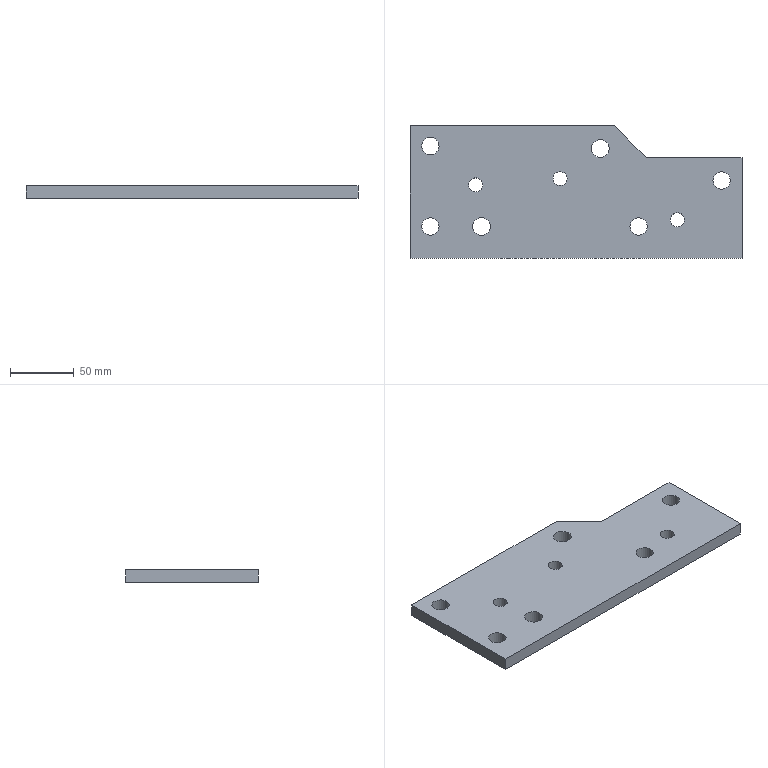Part | STEP file | lll_id114_x_t | 1 solid | 17 faces | box 260 x 104 x 10 mm | volume 236864 mm3 | cylinder 9 | plane 8 | commonest cylinder face diameters 11 x3 13.509 x3 14 x2 13.5 x1
STEP:
#1=CARTESIAN_POINT('',(832.25,-19.75,92.5));
#2=VERTEX_POINT('',#1);
#3=CARTESIAN_POINT('',(825.5,-19.75,92.5));
#4=DIRECTION('',(0.,0.,1.));
#5=DIRECTION('',(1.,0.,0.));
#6=AXIS2_PLACEMENT_3D('',#3,#4,#5);
#7=CIRCLE('',#6,6.75);
#8=EDGE_CURVE('',#2,#2,#7,.T.);
#9=ORIENTED_EDGE('',*,*,#8,.T.);
#10=EDGE_LOOP('',(#9));
#11=FACE_BOUND('',#10,.T.);
#12=CARTESIAN_POINT('',(741.5,23.25,92.5));
#13=VERTEX_POINT('',#12);
#14=CARTESIAN_POINT('',(766.5,-1.75,92.5));
#15=VERTEX_POINT('',#14);
#16=CARTESIAN_POINT('',(734.,30.75,92.5));
#17=DIRECTION('',(0.7071,-0.7071,0.));
#18=VECTOR('',#17,1.);
#19=LINE('',#16,#18);
#20=EDGE_CURVE('',#13,#15,#19,.T.);
#21=ORIENTED_EDGE('',*,*,#20,.T.);
#22=CARTESIAN_POINT('',(841.5,-1.75,92.5));
#23=VERTEX_POINT('',#22);
#24=CARTESIAN_POINT('',(841.5,-1.75,92.5));
#25=DIRECTION('',(-1.,0.,0.));
#26=VECTOR('',#25,1.);
#27=LINE('',#24,#26);
#28=EDGE_CURVE('',#23,#15,#27,.T.);
#29=ORIENTED_EDGE('',*,*,#28,.F.);
#30=CARTESIAN_POINT('',(841.5,-80.75,92.5));
#31=VERTEX_POINT('',#30);
#32=CARTESIAN_POINT('',(841.5,-1.75,92.5));
#33=DIRECTION('',(0.,-1.,0.));
#34=VECTOR('',#33,1.);
#35=LINE('',#32,#34);
#36=EDGE_CURVE('',#23,#31,#35,.T.);
#37=ORIENTED_EDGE('',*,*,#36,.T.);
#38=CARTESIAN_POINT('',(581.5,-80.75,92.5));
#39=VERTEX_POINT('',#38);
#40=CARTESIAN_POINT('',(679.,-80.75,92.5));
#41=DIRECTION('',(1.,0.,0.));
#42=VECTOR('',#41,1.);
#43=LINE('',#40,#42);
#44=EDGE_CURVE('',#39,#31,#43,.T.);
#45=ORIENTED_EDGE('',*,*,#44,.F.);
#46=CARTESIAN_POINT('',(581.5,23.25,92.5));
#47=VERTEX_POINT('',#46);
#48=CARTESIAN_POINT('',(581.5,-24.25,92.5));
#49=DIRECTION('',(0.,-1.,0.));
#50=VECTOR('',#49,1.);
#51=LINE('',#48,#50);
#52=EDGE_CURVE('',#47,#39,#51,.T.);
#53=ORIENTED_EDGE('',*,*,#52,.F.);
#54=CARTESIAN_POINT('',(679.,23.25,92.5));
#55=DIRECTION('',(-1.,0.,0.));
#56=VECTOR('',#55,1.);
#57=LINE('',#54,#56);
#58=EDGE_CURVE('',#13,#47,#57,.T.);
#59=ORIENTED_EDGE('',*,*,#58,.F.);
#60=EDGE_LOOP('',(#21,#29,#37,#45,#53,#59));
#61=FACE_BOUND('',#60,.T.);
#62=CARTESIAN_POINT('',(693.5,-18.25,92.5));
#63=VERTEX_POINT('',#62);
#64=CARTESIAN_POINT('',(699.,-18.25,92.5));
#65=DIRECTION('',(0.,0.,1.));
#66=DIRECTION('',(-1.,0.,0.));
#67=AXIS2_PLACEMENT_3D('',#64,#65,#66);
#68=CIRCLE('',#67,5.5);
#69=EDGE_CURVE('',#63,#63,#68,.T.);
#70=ORIENTED_EDGE('',*,*,#69,.T.);
#71=EDGE_LOOP('',(#70));
#72=FACE_BOUND('',#71,.T.);
#73=CARTESIAN_POINT('',(723.5,5.25,92.5));
#74=VERTEX_POINT('',#73);
#75=CARTESIAN_POINT('',(730.5,5.25,92.5));
#76=DIRECTION('',(0.,0.,1.));
#77=DIRECTION('',(-1.,0.,0.));
#78=AXIS2_PLACEMENT_3D('',#75,#76,#77);
#79=CIRCLE('',#78,7.);
#80=EDGE_CURVE('',#74,#74,#79,.T.);
#81=ORIENTED_EDGE('',*,*,#80,.T.);
#82=EDGE_LOOP('',(#81));
#83=FACE_BOUND('',#82,.T.);
#84=CARTESIAN_POINT('',(590.745,7.25,92.5));
#85=VERTEX_POINT('',#84);
#86=CARTESIAN_POINT('',(597.5,7.25,92.5));
#87=DIRECTION('',(0.,0.,1.));
#88=DIRECTION('',(-1.,0.,0.));
#89=AXIS2_PLACEMENT_3D('',#86,#87,#88);
#90=CIRCLE('',#89,6.755);
#91=EDGE_CURVE('',#85,#85,#90,.T.);
#92=ORIENTED_EDGE('',*,*,#91,.T.);
#93=EDGE_LOOP('',(#92));
#94=FACE_BOUND('',#93,.T.);
#95=CARTESIAN_POINT('',(590.745,-55.75,92.5));
#96=VERTEX_POINT('',#95);
#97=CARTESIAN_POINT('',(597.5,-55.75,92.5));
#98=DIRECTION('',(0.,0.,1.));
#99=DIRECTION('',(-1.,0.,0.));
#100=AXIS2_PLACEMENT_3D('',#97,#98,#99);
#101=CIRCLE('',#100,6.755);
#102=EDGE_CURVE('',#96,#96,#101,.T.);
#103=ORIENTED_EDGE('',*,*,#102,.T.);
#104=EDGE_LOOP('',(#103));
#105=FACE_BOUND('',#104,.T.);
#106=CARTESIAN_POINT('',(753.745,-55.75,92.5));
#107=VERTEX_POINT('',#106);
#108=CARTESIAN_POINT('',(760.5,-55.75,92.5));
#109=DIRECTION('',(0.,0.,1.));
#110=DIRECTION('',(-1.,0.,0.));
#111=AXIS2_PLACEMENT_3D('',#108,#109,#110);
#112=CIRCLE('',#111,6.755);
#113=EDGE_CURVE('',#107,#107,#112,.T.);
#114=ORIENTED_EDGE('',*,*,#113,.T.);
#115=EDGE_LOOP('',(#114));
#116=FACE_BOUND('',#115,.T.);
#117=CARTESIAN_POINT('',(630.5,-55.75,92.5));
#118=VERTEX_POINT('',#117);
#119=CARTESIAN_POINT('',(637.5,-55.75,92.5));
#120=DIRECTION('',(0.,0.,1.));
#121=DIRECTION('',(-1.,0.,0.));
#122=AXIS2_PLACEMENT_3D('',#119,#120,#121);
#123=CIRCLE('',#122,7.);
#124=EDGE_CURVE('',#118,#118,#123,.T.);
#125=ORIENTED_EDGE('',*,*,#124,.T.);
#126=EDGE_LOOP('',(#125));
#127=FACE_BOUND('',#126,.T.);
#128=CARTESIAN_POINT('',(627.5,-23.25,92.5));
#129=VERTEX_POINT('',#128);
#130=CARTESIAN_POINT('',(633.,-23.25,92.5));
#131=DIRECTION('',(0.,0.,1.));
#132=DIRECTION('',(-1.,0.,0.));
#133=AXIS2_PLACEMENT_3D('',#130,#131,#132);
#134=CIRCLE('',#133,5.5);
#135=EDGE_CURVE('',#129,#129,#134,.T.);
#136=ORIENTED_EDGE('',*,*,#135,.T.);
#137=EDGE_LOOP('',(#136));
#138=FACE_BOUND('',#137,.T.);
#139=CARTESIAN_POINT('',(796.273,-50.5,92.5));
#140=VERTEX_POINT('',#139);
#141=CARTESIAN_POINT('',(790.773,-50.5,92.5));
#142=DIRECTION('',(0.,0.,1.));
#143=DIRECTION('',(1.,0.,0.));
#144=AXIS2_PLACEMENT_3D('',#141,#142,#143);
#145=CIRCLE('',#144,5.5);
#146=EDGE_CURVE('',#140,#140,#145,.T.);
#147=ORIENTED_EDGE('',*,*,#146,.T.);
#148=EDGE_LOOP('',(#147));
#149=FACE_BOUND('',#148,.T.);
#150=CARTESIAN_POINT('',(679.,-24.25,92.5));
#151=DIRECTION('',(0.,0.,-1.));
#152=DIRECTION('',(1.,0.,0.));
#153=AXIS2_PLACEMENT_3D('',#150,#151,#152);
#154=PLANE('',#153);
#155=ADVANCED_FACE('',(#11,#61,#72,#83,#94,#105,#116,#127,#138,#149),#154,.T.);
#156=CARTESIAN_POINT('',(581.5,23.25,102.5));
#157=VERTEX_POINT('',#156);
#158=CARTESIAN_POINT('',(741.5,23.25,102.5));
#159=VERTEX_POINT('',#158);
#160=CARTESIAN_POINT('',(679.,23.25,102.5));
#161=DIRECTION('',(1.,0.,0.));
#162=VECTOR('',#161,1.);
#163=LINE('',#160,#162);
#164=EDGE_CURVE('',#157,#159,#163,.T.);
#165=ORIENTED_EDGE('',*,*,#164,.T.);
#166=CARTESIAN_POINT('',(741.5,23.25,92.5));
#167=DIRECTION('',(0.,0.,-1.));
#168=VECTOR('',#167,1.);
#169=LINE('',#166,#168);
#170=EDGE_CURVE('',#159,#13,#169,.T.);
#171=ORIENTED_EDGE('',*,*,#170,.T.);
#172=ORIENTED_EDGE('',*,*,#58,.T.);
#173=CARTESIAN_POINT('',(581.5,23.25,92.5));
#174=DIRECTION('',(0.,0.,1.));
#175=VECTOR('',#174,1.);
#176=LINE('',#173,#175);
#177=EDGE_CURVE('',#47,#157,#176,.T.);
#178=ORIENTED_EDGE('',*,*,#177,.T.);
#179=EDGE_LOOP('',(#165,#171,#172,#178));
#180=FACE_OUTER_BOUND('',#179,.T.);
#181=CARTESIAN_POINT('',(679.,23.25,92.5));
#182=DIRECTION('',(0.,1.,0.));
#183=DIRECTION('',(0.,0.,-1.));
#184=AXIS2_PLACEMENT_3D('',#181,#182,#183);
#185=PLANE('',#184);
#186=ADVANCED_FACE('',(#180),#185,.T.);
#187=CARTESIAN_POINT('',(841.5,-80.75,102.5));
#188=VERTEX_POINT('',#187);
#189=CARTESIAN_POINT('',(581.5,-80.75,102.5));
#190=VERTEX_POINT('',#189);
#191=CARTESIAN_POINT('',(741.5,-80.75,102.5));
#192=DIRECTION('',(-1.,0.,0.));
#193=VECTOR('',#192,1.);
#194=LINE('',#191,#193);
#195=EDGE_CURVE('',#188,#190,#194,.T.);
#196=ORIENTED_EDGE('',*,*,#195,.T.);
#197=CARTESIAN_POINT('',(581.5,-80.75,92.5));
#198=DIRECTION('',(0.,0.,1.));
#199=VECTOR('',#198,1.);
#200=LINE('',#197,#199);
#201=EDGE_CURVE('',#39,#190,#200,.T.);
#202=ORIENTED_EDGE('',*,*,#201,.F.);
#203=ORIENTED_EDGE('',*,*,#44,.T.);
#204=CARTESIAN_POINT('',(841.5,-80.75,102.5));
#205=DIRECTION('',(0.,0.,-1.));
#206=VECTOR('',#205,1.);
#207=LINE('',#204,#206);
#208=EDGE_CURVE('',#188,#31,#207,.T.);
#209=ORIENTED_EDGE('',*,*,#208,.F.);
#210=EDGE_LOOP('',(#196,#202,#203,#209));
#211=FACE_OUTER_BOUND('',#210,.T.);
#212=CARTESIAN_POINT('',(679.,-80.75,92.5));
#213=DIRECTION('',(0.,-1.,0.));
#214=DIRECTION('',(0.,0.,1.));
#215=AXIS2_PLACEMENT_3D('',#212,#213,#214);
#216=PLANE('',#215);
#217=ADVANCED_FACE('',(#211),#216,.T.);
#218=CARTESIAN_POINT('',(581.5,-24.25,102.5));
#219=DIRECTION('',(0.,-1.,0.));
#220=VECTOR('',#219,1.);
#221=LINE('',#218,#220);
#222=EDGE_CURVE('',#157,#190,#221,.T.);
#223=ORIENTED_EDGE('',*,*,#222,.F.);
#224=ORIENTED_EDGE('',*,*,#177,.F.);
#225=ORIENTED_EDGE('',*,*,#52,.T.);
#226=ORIENTED_EDGE('',*,*,#201,.T.);
#227=EDGE_LOOP('',(#223,#224,#225,#226));
#228=FACE_OUTER_BOUND('',#227,.T.);
#229=CARTESIAN_POINT('',(581.5,-24.25,92.5));
#230=DIRECTION('',(-1.,0.,0.));
#231=DIRECTION('',(0.,0.,-1.));
#232=AXIS2_PLACEMENT_3D('',#229,#230,#231);
#233=PLANE('',#232);
#234=ADVANCED_FACE('',(#228),#233,.T.);
#235=CARTESIAN_POINT('',(590.745,-55.75,102.5));
#236=VERTEX_POINT('',#235);
#237=CARTESIAN_POINT('',(597.5,-55.75,102.5));
#238=DIRECTION('',(0.,0.,1.));
#239=DIRECTION('',(-1.,0.,0.));
#240=AXIS2_PLACEMENT_3D('',#237,#238,#239);
#241=CIRCLE('',#240,6.755);
#242=EDGE_CURVE('',#236,#236,#241,.T.);
#243=ORIENTED_EDGE('',*,*,#242,.T.);
#244=EDGE_LOOP('',(#243));
#245=FACE_BOUND('',#244,.T.);
#246=ORIENTED_EDGE('',*,*,#102,.F.);
#247=EDGE_LOOP('',(#246));
#248=FACE_BOUND('',#247,.T.);
#249=CARTESIAN_POINT('',(597.5,-55.75,92.5));
#250=DIRECTION('',(0.,0.,1.));
#251=DIRECTION('',(-1.,0.,0.));
#252=AXIS2_PLACEMENT_3D('',#249,#250,#251);
#253=CYLINDRICAL_SURFACE('',#252,6.755);
#254=ADVANCED_FACE('',(#245,#248),#253,.F.);
#255=CARTESIAN_POINT('',(590.745,7.25,102.5));
#256=VERTEX_POINT('',#255);
#257=CARTESIAN_POINT('',(597.5,7.25,102.5));
#258=DIRECTION('',(0.,0.,1.));
#259=DIRECTION('',(-1.,0.,0.));
#260=AXIS2_PLACEMENT_3D('',#257,#258,#259);
#261=CIRCLE('',#260,6.755);
#262=EDGE_CURVE('',#256,#256,#261,.T.);
#263=ORIENTED_EDGE('',*,*,#262,.T.);
#264=EDGE_LOOP('',(#263));
#265=FACE_BOUND('',#264,.T.);
#266=ORIENTED_EDGE('',*,*,#91,.F.);
#267=EDGE_LOOP('',(#266));
#268=FACE_BOUND('',#267,.T.);
#269=CARTESIAN_POINT('',(597.5,7.25,92.5));
#270=DIRECTION('',(0.,0.,1.));
#271=DIRECTION('',(-1.,0.,0.));
#272=AXIS2_PLACEMENT_3D('',#269,#270,#271);
#273=CYLINDRICAL_SURFACE('',#272,6.755);
#274=ADVANCED_FACE('',(#265,#268),#273,.F.);
#275=CARTESIAN_POINT('',(753.745,-55.75,102.5));
#276=VERTEX_POINT('',#275);
#277=CARTESIAN_POINT('',(760.5,-55.75,102.5));
#278=DIRECTION('',(0.,0.,1.));
#279=DIRECTION('',(-1.,0.,0.));
#280=AXIS2_PLACEMENT_3D('',#277,#278,#279);
#281=CIRCLE('',#280,6.755);
#282=EDGE_CURVE('',#276,#276,#281,.T.);
#283=ORIENTED_EDGE('',*,*,#282,.T.);
#284=EDGE_LOOP('',(#283));
#285=FACE_BOUND('',#284,.T.);
#286=ORIENTED_EDGE('',*,*,#113,.F.);
#287=EDGE_LOOP('',(#286));
#288=FACE_BOUND('',#287,.T.);
#289=CARTESIAN_POINT('',(760.5,-55.75,92.5));
#290=DIRECTION('',(0.,0.,1.));
#291=DIRECTION('',(-1.,0.,0.));
#292=AXIS2_PLACEMENT_3D('',#289,#290,#291);
#293=CYLINDRICAL_SURFACE('',#292,6.755);
#294=ADVANCED_FACE('',(#285,#288),#293,.F.);
#295=CARTESIAN_POINT('',(723.5,5.25,102.5));
#296=VERTEX_POINT('',#295);
#297=CARTESIAN_POINT('',(730.5,5.25,102.5));
#298=DIRECTION('',(0.,0.,-1.));
#299=DIRECTION('',(-1.,0.,0.));
#300=AXIS2_PLACEMENT_3D('',#297,#298,#299);
#301=CIRCLE('',#300,7.);
#302=EDGE_CURVE('',#296,#296,#301,.T.);
#303=ORIENTED_EDGE('',*,*,#302,.F.);
#304=EDGE_LOOP('',(#303));
#305=FACE_BOUND('',#304,.T.);
#306=ORIENTED_EDGE('',*,*,#80,.F.);
#307=EDGE_LOOP('',(#306));
#308=FACE_BOUND('',#307,.T.);
#309=CARTESIAN_POINT('',(730.5,5.25,92.5));
#310=DIRECTION('',(0.,0.,1.));
#311=DIRECTION('',(-1.,0.,0.));
#312=AXIS2_PLACEMENT_3D('',#309,#310,#311);
#313=CYLINDRICAL_SURFACE('',#312,7.);
#314=ADVANCED_FACE('',(#305,#308),#313,.F.);
#315=CARTESIAN_POINT('',(630.5,-55.75,102.5));
#316=VERTEX_POINT('',#315);
#317=CARTESIAN_POINT('',(637.5,-55.75,102.5));
#318=DIRECTION('',(0.,0.,1.));
#319=DIRECTION('',(-1.,0.,0.));
#320=AXIS2_PLACEMENT_3D('',#317,#318,#319);
#321=CIRCLE('',#320,7.);
#322=EDGE_CURVE('',#316,#316,#321,.T.);
#323=ORIENTED_EDGE('',*,*,#322,.T.);
#324=EDGE_LOOP('',(#323));
#325=FACE_BOUND('',#324,.T.);
#326=ORIENTED_EDGE('',*,*,#124,.F.);
#327=EDGE_LOOP('',(#326));
#328=FACE_BOUND('',#327,.T.);
#329=CARTESIAN_POINT('',(637.5,-55.75,92.5));
#330=DIRECTION('',(0.,0.,1.));
#331=DIRECTION('',(-1.,0.,0.));
#332=AXIS2_PLACEMENT_3D('',#329,#330,#331);
#333=CYLINDRICAL_SURFACE('',#332,7.);
#334=ADVANCED_FACE('',(#325,#328),#333,.F.);
#335=CARTESIAN_POINT('',(693.5,-18.25,102.5));
#336=VERTEX_POINT('',#335);
#337=CARTESIAN_POINT('',(699.,-18.25,102.5));
#338=DIRECTION('',(0.,0.,1.));
#339=DIRECTION('',(-1.,0.,0.));
#340=AXIS2_PLACEMENT_3D('',#337,#338,#339);
#341=CIRCLE('',#340,5.5);
#342=EDGE_CURVE('',#336,#336,#341,.T.);
#343=ORIENTED_EDGE('',*,*,#342,.T.);
#344=EDGE_LOOP('',(#343));
#345=FACE_BOUND('',#344,.T.);
#346=ORIENTED_EDGE('',*,*,#69,.F.);
#347=EDGE_LOOP('',(#346));
#348=FACE_BOUND('',#347,.T.);
#349=CARTESIAN_POINT('',(699.,-18.25,217.5));
#350=DIRECTION('',(0.,0.,-1.));
#351=DIRECTION('',(-1.,0.,0.));
#352=AXIS2_PLACEMENT_3D('',#349,#350,#351);
#353=CYLINDRICAL_SURFACE('',#352,5.5);
#354=ADVANCED_FACE('',(#345,#348),#353,.F.);
#355=CARTESIAN_POINT('',(627.5,-23.25,102.5));
#356=VERTEX_POINT('',#355);
#357=CARTESIAN_POINT('',(633.,-23.25,102.5));
#358=DIRECTION('',(0.,0.,-1.));
#359=DIRECTION('',(-1.,0.,0.));
#360=AXIS2_PLACEMENT_3D('',#357,#358,#359);
#361=CIRCLE('',#360,5.5);
#362=EDGE_CURVE('',#356,#356,#361,.T.);
#363=ORIENTED_EDGE('',*,*,#362,.F.);
#364=EDGE_LOOP('',(#363));
#365=FACE_BOUND('',#364,.T.);
#366=ORIENTED_EDGE('',*,*,#135,.F.);
#367=EDGE_LOOP('',(#366));
#368=FACE_BOUND('',#367,.T.);
#369=CARTESIAN_POINT('',(633.,-23.25,217.5));
#370=DIRECTION('',(0.,0.,-1.));
#371=DIRECTION('',(-1.,0.,0.));
#372=AXIS2_PLACEMENT_3D('',#369,#370,#371);
#373=CYLINDRICAL_SURFACE('',#372,5.5);
#374=ADVANCED_FACE('',(#365,#368),#373,.F.);
#375=CARTESIAN_POINT('',(785.273,-50.5,102.5));
#376=VERTEX_POINT('',#375);
#377=CARTESIAN_POINT('',(790.773,-50.5,102.5));
#378=DIRECTION('',(0.,0.,-1.));
#379=DIRECTION('',(-1.,0.,0.));
#380=AXIS2_PLACEMENT_3D('',#377,#378,#379);
#381=CIRCLE('',#380,5.5);
#382=EDGE_CURVE('',#376,#376,#381,.T.);
#383=ORIENTED_EDGE('',*,*,#382,.T.);
#384=EDGE_LOOP('',(#383));
#385=FACE_BOUND('',#384,.T.);
#386=CARTESIAN_POINT('',(818.75,-19.75,102.5));
#387=VERTEX_POINT('',#386);
#388=CARTESIAN_POINT('',(825.5,-19.75,102.5));
#389=DIRECTION('',(0.,0.,-1.));
#390=DIRECTION('',(-1.,0.,0.));
#391=AXIS2_PLACEMENT_3D('',#388,#389,#390);
#392=CIRCLE('',#391,6.75);
#393=EDGE_CURVE('',#387,#387,#392,.T.);
#394=ORIENTED_EDGE('',*,*,#393,.T.);
#395=EDGE_LOOP('',(#394));
#396=FACE_BOUND('',#395,.T.);
#397=ORIENTED_EDGE('',*,*,#195,.F.);
#398=CARTESIAN_POINT('',(841.5,-1.75,102.5));
#399=VERTEX_POINT('',#398);
#400=CARTESIAN_POINT('',(841.5,-1.75,102.5));
#401=DIRECTION('',(0.,-1.,0.));
#402=VECTOR('',#401,1.);
#403=LINE('',#400,#402);
#404=EDGE_CURVE('',#399,#188,#403,.T.);
#405=ORIENTED_EDGE('',*,*,#404,.F.);
#406=CARTESIAN_POINT('',(766.5,-1.75,102.5));
#407=VERTEX_POINT('',#406);
#408=CARTESIAN_POINT('',(841.5,-1.75,102.5));
#409=DIRECTION('',(-1.,0.,0.));
#410=VECTOR('',#409,1.);
#411=LINE('',#408,#410);
#412=EDGE_CURVE('',#399,#407,#411,.T.);
#413=ORIENTED_EDGE('',*,*,#412,.T.);
#414=CARTESIAN_POINT('',(776.5,-11.75,102.5));
#415=DIRECTION('',(-0.7071,0.7071,0.));
#416=VECTOR('',#415,1.);
#417=LINE('',#414,#416);
#418=EDGE_CURVE('',#407,#159,#417,.T.);
#419=ORIENTED_EDGE('',*,*,#418,.T.);
#420=ORIENTED_EDGE('',*,*,#164,.F.);
#421=ORIENTED_EDGE('',*,*,#222,.T.);
#422=EDGE_LOOP('',(#397,#405,#413,#419,#420,#421));
#423=FACE_BOUND('',#422,.T.);
#424=ORIENTED_EDGE('',*,*,#242,.F.);
#425=EDGE_LOOP('',(#424));
#426=FACE_BOUND('',#425,.T.);
#427=ORIENTED_EDGE('',*,*,#282,.F.);
#428=EDGE_LOOP('',(#427));
#429=FACE_BOUND('',#428,.T.);
#430=ORIENTED_EDGE('',*,*,#322,.F.);
#431=EDGE_LOOP('',(#430));
#432=FACE_BOUND('',#431,.T.);
#433=ORIENTED_EDGE('',*,*,#342,.F.);
#434=EDGE_LOOP('',(#433));
#435=FACE_BOUND('',#434,.T.);
#436=ORIENTED_EDGE('',*,*,#362,.T.);
#437=EDGE_LOOP('',(#436));
#438=FACE_BOUND('',#437,.T.);
#439=ORIENTED_EDGE('',*,*,#302,.T.);
#440=EDGE_LOOP('',(#439));
#441=FACE_BOUND('',#440,.T.);
#442=ORIENTED_EDGE('',*,*,#262,.F.);
#443=EDGE_LOOP('',(#442));
#444=FACE_BOUND('',#443,.T.);
#445=CARTESIAN_POINT('',(741.5,-0.002299,102.5));
#446=DIRECTION('',(0.,0.,-1.));
#447=DIRECTION('',(-1.,0.,0.));
#448=AXIS2_PLACEMENT_3D('',#445,#446,#447);
#449=PLANE('',#448);
#450=ADVANCED_FACE('',(#385,#396,#423,#426,#429,#432,#435,#438,#441,#444),#449,.F.);
#451=ORIENTED_EDGE('',*,*,#20,.F.);
#452=ORIENTED_EDGE('',*,*,#170,.F.);
#453=ORIENTED_EDGE('',*,*,#418,.F.);
#454=CARTESIAN_POINT('',(766.5,-1.75,102.5));
#455=DIRECTION('',(0.,0.,-1.));
#456=VECTOR('',#455,1.);
#457=LINE('',#454,#456);
#458=EDGE_CURVE('',#407,#15,#457,.T.);
#459=ORIENTED_EDGE('',*,*,#458,.T.);
#460=EDGE_LOOP('',(#451,#452,#453,#459));
#461=FACE_OUTER_BOUND('',#460,.T.);
#462=CARTESIAN_POINT('',(776.5,-11.75,92.5));
#463=DIRECTION('',(-0.7071,-0.7071,0.));
#464=DIRECTION('',(0.,0.,1.));
#465=AXIS2_PLACEMENT_3D('',#462,#463,#464);
#466=PLANE('',#465);
#467=ADVANCED_FACE('',(#461),#466,.F.);
#468=ORIENTED_EDGE('',*,*,#28,.T.);
#469=ORIENTED_EDGE('',*,*,#458,.F.);
#470=ORIENTED_EDGE('',*,*,#412,.F.);
#471=CARTESIAN_POINT('',(841.5,-1.75,102.5));
#472=DIRECTION('',(0.,0.,-1.));
#473=VECTOR('',#472,1.);
#474=LINE('',#471,#473);
#475=EDGE_CURVE('',#399,#23,#474,.T.);
#476=ORIENTED_EDGE('',*,*,#475,.T.);
#477=EDGE_LOOP('',(#468,#469,#470,#476));
#478=FACE_OUTER_BOUND('',#477,.T.);
#479=CARTESIAN_POINT('',(841.5,-1.75,102.5));
#480=DIRECTION('',(0.,-1.,0.));
#481=DIRECTION('',(0.,0.,-1.));
#482=AXIS2_PLACEMENT_3D('',#479,#480,#481);
#483=PLANE('',#482);
#484=ADVANCED_FACE('',(#478),#483,.F.);
#485=ORIENTED_EDGE('',*,*,#36,.F.);
#486=ORIENTED_EDGE('',*,*,#475,.F.);
#487=ORIENTED_EDGE('',*,*,#404,.T.);
#488=ORIENTED_EDGE('',*,*,#208,.T.);
#489=EDGE_LOOP('',(#485,#486,#487,#488));
#490=FACE_OUTER_BOUND('',#489,.T.);
#491=CARTESIAN_POINT('',(841.5,-1.75,102.5));
#492=DIRECTION('',(1.,0.,0.));
#493=DIRECTION('',(0.,0.,-1.));
#494=AXIS2_PLACEMENT_3D('',#491,#492,#493);
#495=PLANE('',#494);
#496=ADVANCED_FACE('',(#490),#495,.T.);
#497=ORIENTED_EDGE('',*,*,#8,.F.);
#498=EDGE_LOOP('',(#497));
#499=FACE_BOUND('',#498,.T.);
#500=ORIENTED_EDGE('',*,*,#393,.F.);
#501=EDGE_LOOP('',(#500));
#502=FACE_BOUND('',#501,.T.);
#503=CARTESIAN_POINT('',(825.5,-19.75,92.5));
#504=DIRECTION('',(0.,0.,1.));
#505=DIRECTION('',(1.,0.,0.));
#506=AXIS2_PLACEMENT_3D('',#503,#504,#505);
#507=CYLINDRICAL_SURFACE('',#506,6.75);
#508=ADVANCED_FACE('',(#499,#502),#507,.F.);
#509=ORIENTED_EDGE('',*,*,#146,.F.);
#510=EDGE_LOOP('',(#509));
#511=FACE_BOUND('',#510,.T.);
#512=ORIENTED_EDGE('',*,*,#382,.F.);
#513=EDGE_LOOP('',(#512));
#514=FACE_BOUND('',#513,.T.);
#515=CARTESIAN_POINT('',(790.773,-50.5,92.5));
#516=DIRECTION('',(0.,0.,1.));
#517=DIRECTION('',(1.,0.,0.));
#518=AXIS2_PLACEMENT_3D('',#515,#516,#517);
#519=CYLINDRICAL_SURFACE('',#518,5.5);
#520=ADVANCED_FACE('',(#511,#514),#519,.F.);
#521=CLOSED_SHELL('',(#155,#186,#217,#234,#254,#274,#294,#314,#334,#354,#374,#450,#467,#484,#496,#508,#520));
#522=MANIFOLD_SOLID_BREP('',#521);
#523=(LENGTH_UNIT()NAMED_UNIT(*)SI_UNIT(.MILLI.,.METRE.));
#524=UNCERTAINTY_MEASURE_WITH_UNIT(LENGTH_MEASURE(0.00002),#523,'','');
#525=(NAMED_UNIT(*)PLANE_ANGLE_UNIT()SI_UNIT($,.RADIAN.));
#526=PLANE_ANGLE_MEASURE_WITH_UNIT(PLANE_ANGLE_MEASURE(0.01745),#525);
#527=DIMENSIONAL_EXPONENTS(0.,0.,0.,0.,0.,0.,0.);
#528=(CONVERSION_BASED_UNIT('DEGREE',#526)NAMED_UNIT(#527)PLANE_ANGLE_UNIT());
#529=(NAMED_UNIT(*)SI_UNIT($,.STERADIAN.)SOLID_ANGLE_UNIT());
#530=(GEOMETRIC_REPRESENTATION_CONTEXT(3)GLOBAL_UNCERTAINTY_ASSIGNED_CONTEXT((#524))GLOBAL_UNIT_ASSIGNED_CONTEXT((#523,#528,#529))REPRESENTATION_CONTEXT('',''));
#531=ADVANCED_BREP_SHAPE_REPRESENTATION('',(#522),#530);